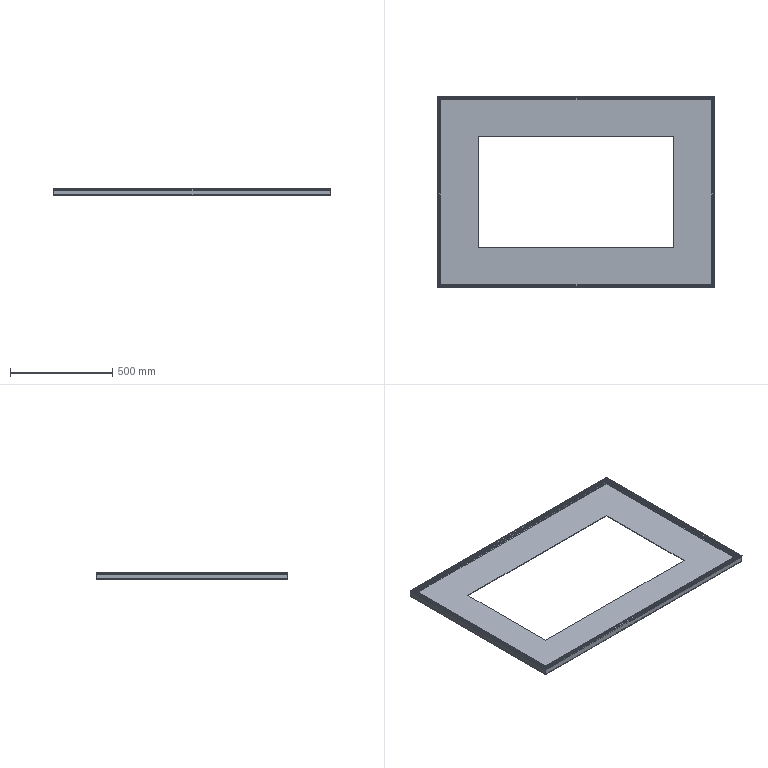Part | SolidWorks | features Cut 1, ICE 1, WeldMemberFeat 1, WeldmentFeature 1 | 5 solids | 98 faces | box 1360 x 940 x 35 mm | volume 2869599 mm3 | plane 90 | cylinder 8 | commonest cylinder face diameters 1 x4 2 x4